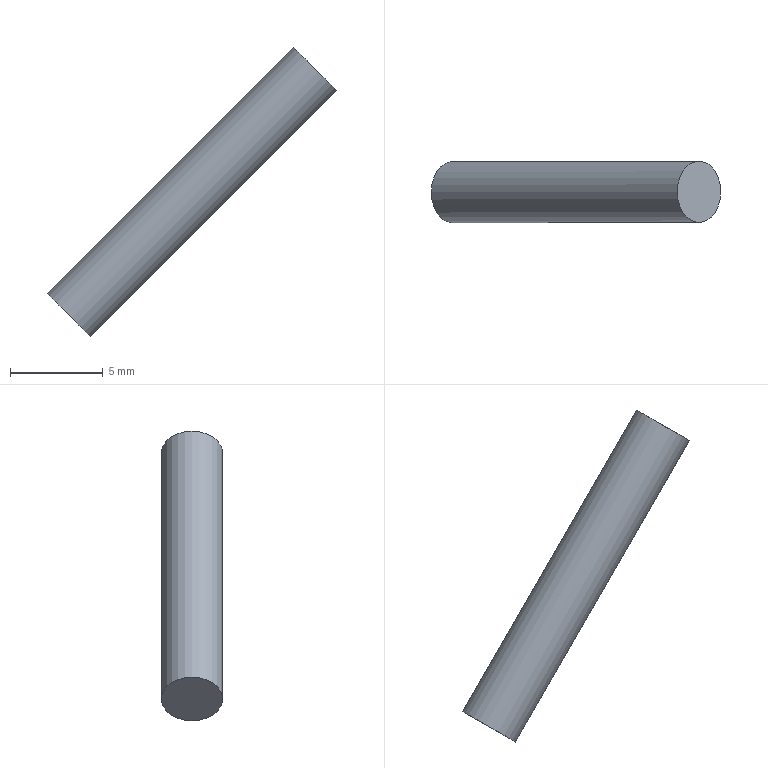Part | STEP file | basic_gh_motor_gh1_13 | 1 solid | 3 faces | box 15.57 x 3.3 x 15.57 mm | volume 160.112 mm3 | plane 2 | cylinder 1 | commonest cylinder face diameters 3.3 x1
STEP:
#1=CARTESIAN_POINT('',(-71.248,136.55,7.785));
#2=VERTEX_POINT('',#1);
#3=CARTESIAN_POINT('',(-70.081,136.55,6.619));
#4=DIRECTION('',(0.7071,0.,0.7071));
#5=DIRECTION('',(0.7071,0.,-0.7071));
#6=AXIS2_PLACEMENT_3D('',#3,#4,#5);
#7=CIRCLE('',#6,1.65);
#8=EDGE_CURVE('',#2,#2,#7,.T.);
#9=ORIENTED_EDGE('',*,*,#8,.F.);
#10=CARTESIAN_POINT('',(-84.485,136.55,-5.452));
#11=VERTEX_POINT('',#10);
#12=CARTESIAN_POINT('',(-77.867,136.55,1.167));
#13=DIRECTION('',(-0.7071,0.,-0.7071));
#14=VECTOR('',#13,1.65);
#15=LINE('',#12,#14);
#16=EDGE_CURVE('',#2,#11,#15,.T.);
#17=ORIENTED_EDGE('',*,*,#16,.T.);
#18=CARTESIAN_POINT('',(-83.319,136.55,-6.619));
#19=DIRECTION('',(-0.7071,0.,-0.7071));
#20=DIRECTION('',(0.7071,0.,-0.7071));
#21=AXIS2_PLACEMENT_3D('',#18,#19,#20);
#22=CIRCLE('',#21,1.65);
#23=EDGE_CURVE('',#11,#11,#22,.T.);
#24=ORIENTED_EDGE('',*,*,#23,.F.);
#25=ORIENTED_EDGE('',*,*,#16,.F.);
#26=EDGE_LOOP('',(#9,#17,#24,#25));
#27=FACE_OUTER_BOUND('',#26,.T.);
#28=CARTESIAN_POINT('',(-76.7,136.55,0.));
#29=DIRECTION('',(0.7071,0.,0.7071));
#30=DIRECTION('',(0.7071,0.,-0.7071));
#31=AXIS2_PLACEMENT_3D('',#28,#29,#30);
#32=CYLINDRICAL_SURFACE('',#31,1.65);
#33=ADVANCED_FACE('',(#27),#32,.T.);
#34=ORIENTED_EDGE('',*,*,#23,.T.);
#35=EDGE_LOOP('',(#34));
#36=FACE_OUTER_BOUND('',#35,.T.);
#37=CARTESIAN_POINT('',(-83.319,136.55,-6.619));
#38=DIRECTION('',(-0.7071,0.,-0.7071));
#39=DIRECTION('',(-0.7071,0.,0.7071));
#40=AXIS2_PLACEMENT_3D('',#37,#38,#39);
#41=PLANE('',#40);
#42=ADVANCED_FACE('',(#36),#41,.T.);
#43=ORIENTED_EDGE('',*,*,#8,.T.);
#44=EDGE_LOOP('',(#43));
#45=FACE_OUTER_BOUND('',#44,.T.);
#46=CARTESIAN_POINT('',(-70.081,136.55,6.619));
#47=DIRECTION('',(0.7071,0.,0.7071));
#48=DIRECTION('',(0.7071,0.,-0.7071));
#49=AXIS2_PLACEMENT_3D('',#46,#47,#48);
#50=PLANE('',#49);
#51=ADVANCED_FACE('',(#45),#50,.T.);
#52=CLOSED_SHELL('',(#33,#42,#51));
#53=MANIFOLD_SOLID_BREP('',#52);
#54=(LENGTH_UNIT()NAMED_UNIT(*)SI_UNIT(.MILLI.,.METRE.));
#55=UNCERTAINTY_MEASURE_WITH_UNIT(LENGTH_MEASURE(0.01),#54,'','');
#56=(NAMED_UNIT(*)PLANE_ANGLE_UNIT()SI_UNIT($,.RADIAN.));
#57=(NAMED_UNIT(*)SI_UNIT($,.STERADIAN.)SOLID_ANGLE_UNIT());
#58=(GEOMETRIC_REPRESENTATION_CONTEXT(3)GLOBAL_UNCERTAINTY_ASSIGNED_CONTEXT((#55))GLOBAL_UNIT_ASSIGNED_CONTEXT((#54,#56,#57))REPRESENTATION_CONTEXT('',''));
#59=ADVANCED_BREP_SHAPE_REPRESENTATION('',(#53),#58);